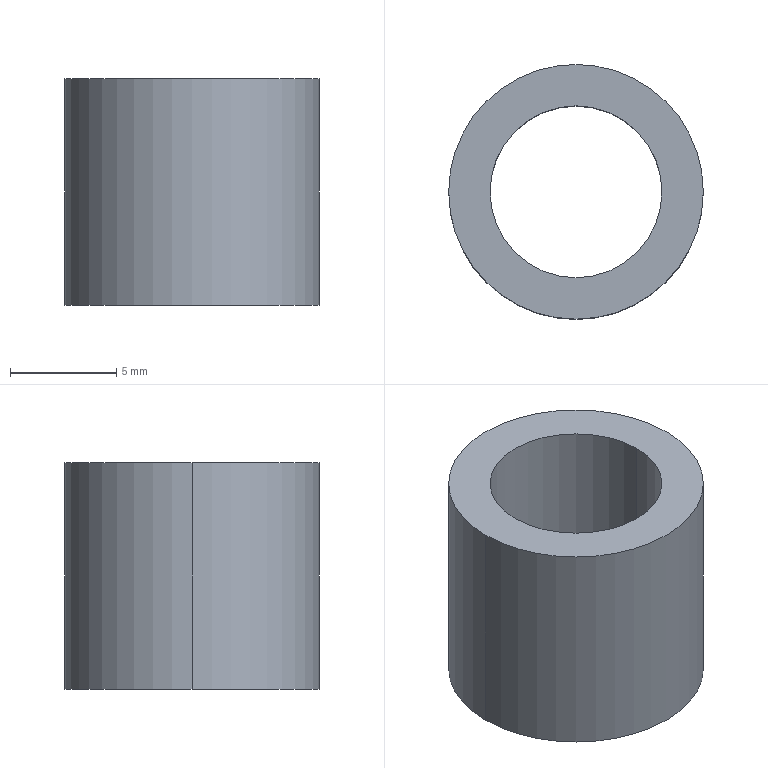Part | SolidWorks | features Extrusion 1 | 1 solid | 6 faces | box 12 x 12 x 10.677 mm | volume 657.35 mm3 | cylinder 4 | plane 2 | commonest cylinder face diameters 8.1 x2 12 x2
STEP:
#1=CARTESIAN_POINT('',(5.95,-61.753,10.677));
#2=VERTEX_POINT('',#1);
#3=CARTESIAN_POINT('',(14.05,-61.753,10.677));
#4=VERTEX_POINT('',#3);
#5=CARTESIAN_POINT('',(10.,-61.753,10.677));
#6=DIRECTION('',(0.,0.,1.));
#7=DIRECTION('',(1.,0.,0.));
#8=AXIS2_PLACEMENT_3D('',#5,#6,#7);
#9=CIRCLE('',#8,4.05);
#10=EDGE_CURVE('',#2,#4,#9,.T.);
#11=ORIENTED_EDGE('',*,*,#10,.T.);
#12=CARTESIAN_POINT('',(14.05,-61.753,0.));
#13=VERTEX_POINT('',#12);
#14=CARTESIAN_POINT('',(14.05,-61.753,27.647));
#15=DIRECTION('',(0.,0.,-1.));
#16=VECTOR('',#15,1000.);
#17=LINE('',#14,#16);
#18=EDGE_CURVE('',#4,#13,#17,.T.);
#19=ORIENTED_EDGE('',*,*,#18,.T.);
#20=CARTESIAN_POINT('',(5.95,-61.753,0.));
#21=VERTEX_POINT('',#20);
#22=CARTESIAN_POINT('',(10.,-61.753,0.));
#23=DIRECTION('',(0.,0.,1.));
#24=DIRECTION('',(1.,0.,0.));
#25=AXIS2_PLACEMENT_3D('',#22,#23,#24);
#26=CIRCLE('',#25,4.05);
#27=EDGE_CURVE('',#21,#13,#26,.T.);
#28=ORIENTED_EDGE('',*,*,#27,.F.);
#29=CARTESIAN_POINT('',(5.95,-61.753,27.647));
#30=DIRECTION('',(0.,0.,-1.));
#31=VECTOR('',#30,1000.);
#32=LINE('',#29,#31);
#33=EDGE_CURVE('',#2,#21,#32,.T.);
#34=ORIENTED_EDGE('',*,*,#33,.F.);
#35=EDGE_LOOP('',(#11,#19,#28,#34));
#36=FACE_OUTER_BOUND('',#35,.T.);
#37=CARTESIAN_POINT('',(10.,-61.753,27.647));
#38=DIRECTION('',(0.,0.,-1.));
#39=DIRECTION('',(-1.,0.,0.));
#40=AXIS2_PLACEMENT_3D('',#37,#38,#39);
#41=CYLINDRICAL_SURFACE('',#40,4.05);
#42=ADVANCED_FACE('',(#36),#41,.F.);
#43=CARTESIAN_POINT('',(16.,-61.753,10.677));
#44=VERTEX_POINT('',#43);
#45=CARTESIAN_POINT('',(4.,-61.753,10.677));
#46=VERTEX_POINT('',#45);
#47=CARTESIAN_POINT('',(10.,-61.753,10.677));
#48=DIRECTION('',(0.,0.,1.));
#49=DIRECTION('',(1.,0.,0.));
#50=AXIS2_PLACEMENT_3D('',#47,#48,#49);
#51=CIRCLE('',#50,6.);
#52=EDGE_CURVE('',#44,#46,#51,.T.);
#53=ORIENTED_EDGE('',*,*,#52,.F.);
#54=CARTESIAN_POINT('',(16.,-61.753,0.));
#55=VERTEX_POINT('',#54);
#56=CARTESIAN_POINT('',(16.,-61.753,27.647));
#57=DIRECTION('',(0.,0.,-1.));
#58=VECTOR('',#57,1000.);
#59=LINE('',#56,#58);
#60=EDGE_CURVE('',#44,#55,#59,.T.);
#61=ORIENTED_EDGE('',*,*,#60,.T.);
#62=CARTESIAN_POINT('',(4.,-61.753,0.));
#63=VERTEX_POINT('',#62);
#64=CARTESIAN_POINT('',(10.,-61.753,0.));
#65=DIRECTION('',(0.,0.,1.));
#66=DIRECTION('',(1.,0.,0.));
#67=AXIS2_PLACEMENT_3D('',#64,#65,#66);
#68=CIRCLE('',#67,6.);
#69=EDGE_CURVE('',#55,#63,#68,.T.);
#70=ORIENTED_EDGE('',*,*,#69,.T.);
#71=CARTESIAN_POINT('',(4.,-61.753,27.647));
#72=DIRECTION('',(0.,0.,-1.));
#73=VECTOR('',#72,1000.);
#74=LINE('',#71,#73);
#75=EDGE_CURVE('',#46,#63,#74,.T.);
#76=ORIENTED_EDGE('',*,*,#75,.F.);
#77=EDGE_LOOP('',(#53,#61,#70,#76));
#78=FACE_OUTER_BOUND('',#77,.T.);
#79=CARTESIAN_POINT('',(10.,-61.753,27.647));
#80=DIRECTION('',(0.,0.,-1.));
#81=DIRECTION('',(-1.,0.,0.));
#82=AXIS2_PLACEMENT_3D('',#79,#80,#81);
#83=CYLINDRICAL_SURFACE('',#82,6.);
#84=ADVANCED_FACE('',(#78),#83,.T.);
#85=ORIENTED_EDGE('',*,*,#60,.F.);
#86=CARTESIAN_POINT('',(10.,-61.753,10.677));
#87=DIRECTION('',(0.,0.,1.));
#88=DIRECTION('',(1.,0.,0.));
#89=AXIS2_PLACEMENT_3D('',#86,#87,#88);
#90=CIRCLE('',#89,6.);
#91=EDGE_CURVE('',#46,#44,#90,.T.);
#92=ORIENTED_EDGE('',*,*,#91,.F.);
#93=ORIENTED_EDGE('',*,*,#75,.T.);
#94=CARTESIAN_POINT('',(10.,-61.753,0.));
#95=DIRECTION('',(0.,0.,1.));
#96=DIRECTION('',(1.,0.,0.));
#97=AXIS2_PLACEMENT_3D('',#94,#95,#96);
#98=CIRCLE('',#97,6.);
#99=EDGE_CURVE('',#63,#55,#98,.T.);
#100=ORIENTED_EDGE('',*,*,#99,.T.);
#101=EDGE_LOOP('',(#85,#92,#93,#100));
#102=FACE_OUTER_BOUND('',#101,.T.);
#103=CARTESIAN_POINT('',(10.,-61.753,27.647));
#104=DIRECTION('',(0.,0.,-1.));
#105=DIRECTION('',(-1.,0.,0.));
#106=AXIS2_PLACEMENT_3D('',#103,#104,#105);
#107=CYLINDRICAL_SURFACE('',#106,6.);
#108=ADVANCED_FACE('',(#102),#107,.T.);
#109=ORIENTED_EDGE('',*,*,#99,.F.);
#110=ORIENTED_EDGE('',*,*,#69,.F.);
#111=EDGE_LOOP('',(#109,#110));
#112=FACE_OUTER_BOUND('',#111,.T.);
#113=ORIENTED_EDGE('',*,*,#27,.T.);
#114=CARTESIAN_POINT('',(10.,-61.753,0.));
#115=DIRECTION('',(0.,0.,1.));
#116=DIRECTION('',(1.,0.,0.));
#117=AXIS2_PLACEMENT_3D('',#114,#115,#116);
#118=CIRCLE('',#117,4.05);
#119=EDGE_CURVE('',#13,#21,#118,.T.);
#120=ORIENTED_EDGE('',*,*,#119,.T.);
#121=EDGE_LOOP('',(#113,#120));
#122=FACE_BOUND('',#121,.T.);
#123=CARTESIAN_POINT('',(10.,-61.753,0.));
#124=DIRECTION('',(0.,0.,1.));
#125=DIRECTION('',(1.,0.,0.));
#126=AXIS2_PLACEMENT_3D('',#123,#124,#125);
#127=PLANE('',#126);
#128=ADVANCED_FACE('',(#112,#122),#127,.F.);
#129=ORIENTED_EDGE('',*,*,#18,.F.);
#130=CARTESIAN_POINT('',(10.,-61.753,10.677));
#131=DIRECTION('',(0.,0.,1.));
#132=DIRECTION('',(1.,0.,0.));
#133=AXIS2_PLACEMENT_3D('',#130,#131,#132);
#134=CIRCLE('',#133,4.05);
#135=EDGE_CURVE('',#4,#2,#134,.T.);
#136=ORIENTED_EDGE('',*,*,#135,.T.);
#137=ORIENTED_EDGE('',*,*,#33,.T.);
#138=ORIENTED_EDGE('',*,*,#119,.F.);
#139=EDGE_LOOP('',(#129,#136,#137,#138));
#140=FACE_OUTER_BOUND('',#139,.T.);
#141=CARTESIAN_POINT('',(10.,-61.753,27.647));
#142=DIRECTION('',(0.,0.,-1.));
#143=DIRECTION('',(-1.,0.,0.));
#144=AXIS2_PLACEMENT_3D('',#141,#142,#143);
#145=CYLINDRICAL_SURFACE('',#144,4.05);
#146=ADVANCED_FACE('',(#140),#145,.F.);
#147=ORIENTED_EDGE('',*,*,#10,.F.);
#148=ORIENTED_EDGE('',*,*,#135,.F.);
#149=EDGE_LOOP('',(#147,#148));
#150=FACE_BOUND('',#149,.T.);
#151=ORIENTED_EDGE('',*,*,#91,.T.);
#152=ORIENTED_EDGE('',*,*,#52,.T.);
#153=EDGE_LOOP('',(#151,#152));
#154=FACE_OUTER_BOUND('',#153,.T.);
#155=CARTESIAN_POINT('',(10.,-61.753,10.677));
#156=DIRECTION('',(0.,0.,1.));
#157=DIRECTION('',(-0.969,0.2469,0.));
#158=AXIS2_PLACEMENT_3D('',#155,#156,#157);
#159=PLANE('',#158);
#160=ADVANCED_FACE('',(#150,#154),#159,.T.);
#161=CLOSED_SHELL('',(#42,#84,#108,#128,#146,#160));
#162=MANIFOLD_SOLID_BREP('',#161);
#163=CARTESIAN_POINT('',(0.,0.,0.));
#164=DIRECTION('',(0.,0.,1.));
#165=DIRECTION('',(1.,0.,0.));
#166=AXIS2_PLACEMENT_3D('',#163,#164,#165);
#167=(LENGTH_UNIT()NAMED_UNIT(*)SI_UNIT(.MILLI.,.METRE.));
#168=UNCERTAINTY_MEASURE_WITH_UNIT(LENGTH_MEASURE(0.00001),#167,'','');
#169=(NAMED_UNIT(*)PLANE_ANGLE_UNIT()SI_UNIT($,.RADIAN.));
#170=(NAMED_UNIT(*)SI_UNIT($,.STERADIAN.)SOLID_ANGLE_UNIT());
#171=(GEOMETRIC_REPRESENTATION_CONTEXT(3)GLOBAL_UNCERTAINTY_ASSIGNED_CONTEXT((#168))GLOBAL_UNIT_ASSIGNED_CONTEXT((#167,#169,#170))REPRESENTATION_CONTEXT('',''));
#172=ADVANCED_BREP_SHAPE_REPRESENTATION('',(#162,#166),#171);